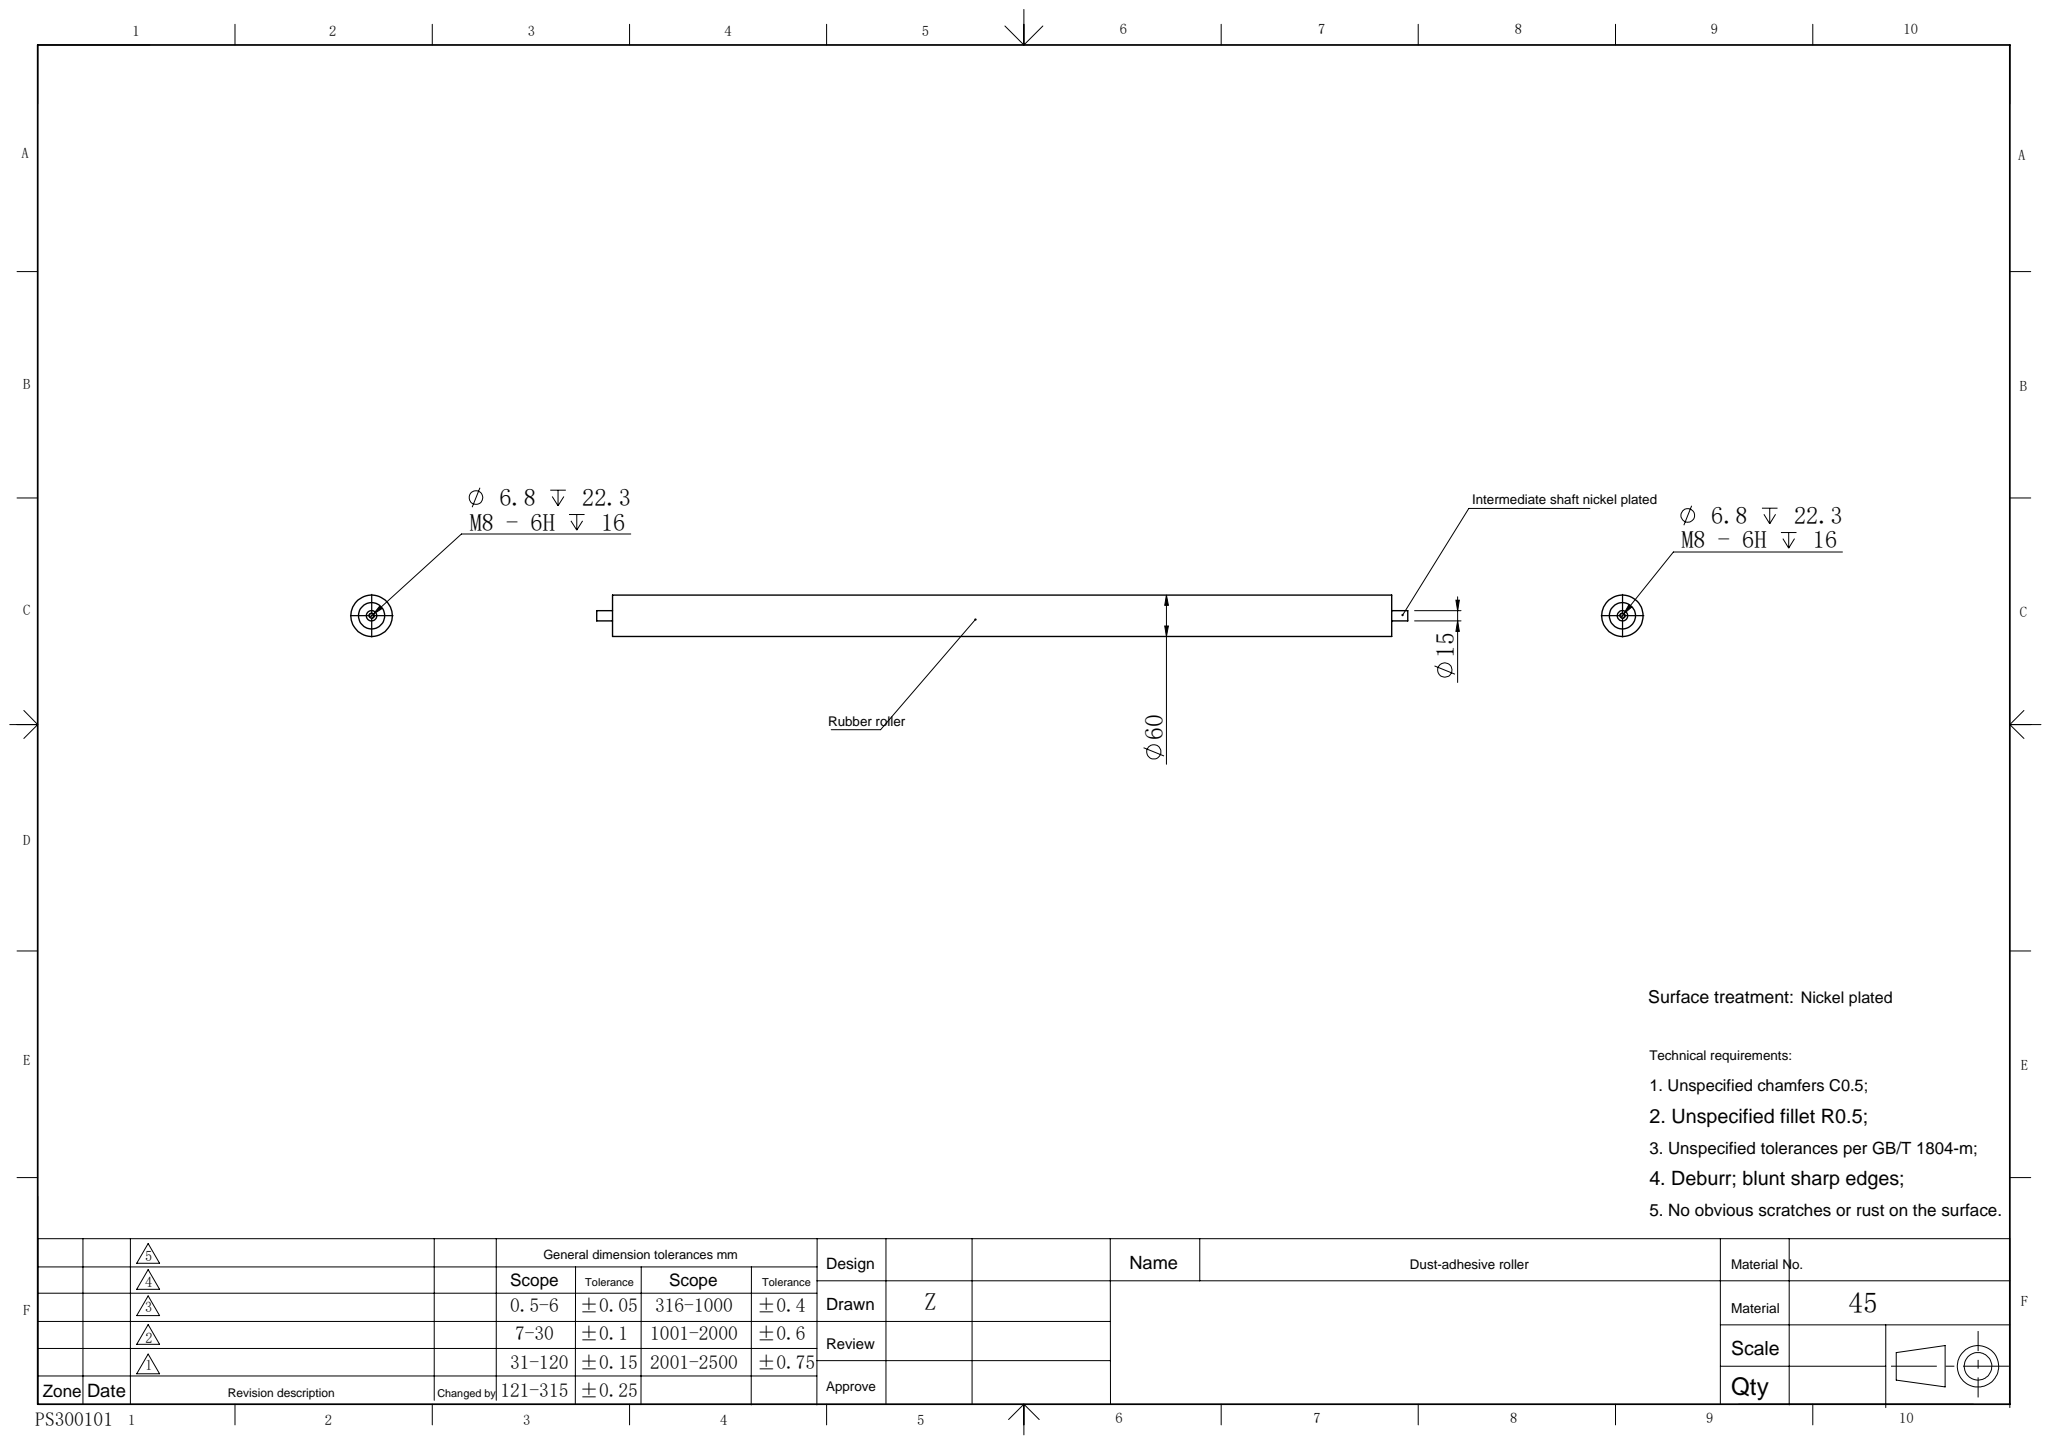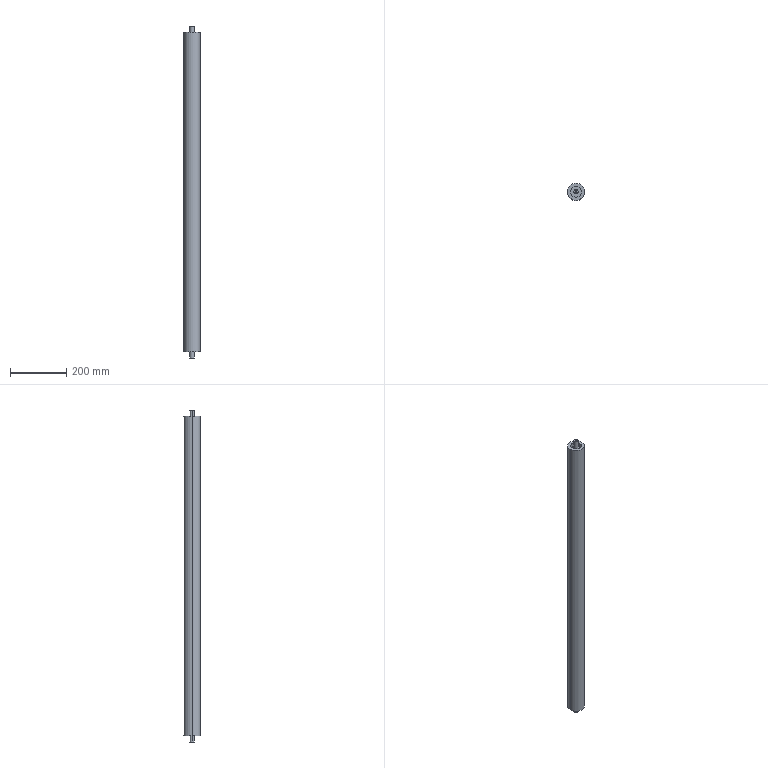Part | SolidWorks | features HoleWzd 2, ICE 2, Extrusion 1 | 2 solids | 24 faces | box 60 x 60 x 1176 mm | volume 3172741 mm3 | cylinder 14 | plane 6 | cone 4 | commonest cylinder face diameters 6.8 x4 15 x4 38 x4 60 x2
STEP:
#1=CARTESIAN_POINT('',(-19.,0.,565.));
#2=VERTEX_POINT('',#1);
#3=CARTESIAN_POINT('',(19.,0.,565.));
#4=VERTEX_POINT('',#3);
#5=CARTESIAN_POINT('',(0.,0.,565.));
#6=DIRECTION('',(0.,0.,1.));
#7=DIRECTION('',(1.,0.,0.));
#8=AXIS2_PLACEMENT_3D('',#5,#6,#7);
#9=CIRCLE('',#8,19.);
#10=EDGE_CURVE('',#2,#4,#9,.T.);
#11=ORIENTED_EDGE('',*,*,#10,.T.);
#12=CARTESIAN_POINT('',(19.,0.,-565.));
#13=VERTEX_POINT('',#12);
#14=CARTESIAN_POINT('',(19.,0.,565.));
#15=DIRECTION('',(0.,0.,-1.));
#16=VECTOR('',#15,1000.);
#17=LINE('',#14,#16);
#18=EDGE_CURVE('',#4,#13,#17,.T.);
#19=ORIENTED_EDGE('',*,*,#18,.T.);
#20=CARTESIAN_POINT('',(-19.,0.,-565.));
#21=VERTEX_POINT('',#20);
#22=CARTESIAN_POINT('',(0.,0.,-565.));
#23=DIRECTION('',(0.,0.,1.));
#24=DIRECTION('',(1.,0.,0.));
#25=AXIS2_PLACEMENT_3D('',#22,#23,#24);
#26=CIRCLE('',#25,19.);
#27=EDGE_CURVE('',#21,#13,#26,.T.);
#28=ORIENTED_EDGE('',*,*,#27,.F.);
#29=CARTESIAN_POINT('',(-19.,0.,565.));
#30=DIRECTION('',(0.,0.,-1.));
#31=VECTOR('',#30,1000.);
#32=LINE('',#29,#31);
#33=EDGE_CURVE('',#2,#21,#32,.T.);
#34=ORIENTED_EDGE('',*,*,#33,.F.);
#35=EDGE_LOOP('',(#11,#19,#28,#34));
#36=FACE_OUTER_BOUND('',#35,.T.);
#37=CARTESIAN_POINT('',(0.,0.,565.));
#38=DIRECTION('',(0.,0.,-1.));
#39=DIRECTION('',(-1.,0.,0.));
#40=AXIS2_PLACEMENT_3D('',#37,#38,#39);
#41=CYLINDRICAL_SURFACE('',#40,19.);
#42=ADVANCED_FACE('',(#36),#41,.F.);
#43=CARTESIAN_POINT('',(30.,0.,565.));
#44=VERTEX_POINT('',#43);
#45=CARTESIAN_POINT('',(-30.,0.,565.));
#46=VERTEX_POINT('',#45);
#47=CARTESIAN_POINT('',(0.,0.,565.));
#48=DIRECTION('',(0.,0.,1.));
#49=DIRECTION('',(1.,0.,0.));
#50=AXIS2_PLACEMENT_3D('',#47,#48,#49);
#51=CIRCLE('',#50,30.);
#52=EDGE_CURVE('',#44,#46,#51,.T.);
#53=ORIENTED_EDGE('',*,*,#52,.F.);
#54=CARTESIAN_POINT('',(30.,0.,-565.));
#55=VERTEX_POINT('',#54);
#56=CARTESIAN_POINT('',(30.,0.,565.));
#57=DIRECTION('',(0.,0.,-1.));
#58=VECTOR('',#57,1000.);
#59=LINE('',#56,#58);
#60=EDGE_CURVE('',#44,#55,#59,.T.);
#61=ORIENTED_EDGE('',*,*,#60,.T.);
#62=CARTESIAN_POINT('',(-30.,0.,-565.));
#63=VERTEX_POINT('',#62);
#64=CARTESIAN_POINT('',(0.,0.,-565.));
#65=DIRECTION('',(0.,0.,1.));
#66=DIRECTION('',(1.,0.,0.));
#67=AXIS2_PLACEMENT_3D('',#64,#65,#66);
#68=CIRCLE('',#67,30.);
#69=EDGE_CURVE('',#55,#63,#68,.T.);
#70=ORIENTED_EDGE('',*,*,#69,.T.);
#71=CARTESIAN_POINT('',(-30.,0.,565.));
#72=DIRECTION('',(0.,0.,-1.));
#73=VECTOR('',#72,1000.);
#74=LINE('',#71,#73);
#75=EDGE_CURVE('',#46,#63,#74,.T.);
#76=ORIENTED_EDGE('',*,*,#75,.F.);
#77=EDGE_LOOP('',(#53,#61,#70,#76));
#78=FACE_OUTER_BOUND('',#77,.T.);
#79=CARTESIAN_POINT('',(0.,0.,565.));
#80=DIRECTION('',(0.,0.,-1.));
#81=DIRECTION('',(-1.,0.,0.));
#82=AXIS2_PLACEMENT_3D('',#79,#80,#81);
#83=CYLINDRICAL_SURFACE('',#82,30.);
#84=ADVANCED_FACE('',(#78),#83,.T.);
#85=CARTESIAN_POINT('',(0.,0.,565.));
#86=DIRECTION('',(0.,0.,1.));
#87=DIRECTION('',(1.,0.,0.));
#88=AXIS2_PLACEMENT_3D('',#85,#86,#87);
#89=CIRCLE('',#88,30.);
#90=EDGE_CURVE('',#46,#44,#89,.T.);
#91=ORIENTED_EDGE('',*,*,#90,.T.);
#92=ORIENTED_EDGE('',*,*,#52,.T.);
#93=EDGE_LOOP('',(#91,#92));
#94=FACE_OUTER_BOUND('',#93,.T.);
#95=ORIENTED_EDGE('',*,*,#10,.F.);
#96=CARTESIAN_POINT('',(0.,0.,565.));
#97=DIRECTION('',(0.,0.,1.));
#98=DIRECTION('',(1.,0.,0.));
#99=AXIS2_PLACEMENT_3D('',#96,#97,#98);
#100=CIRCLE('',#99,19.);
#101=EDGE_CURVE('',#4,#2,#100,.T.);
#102=ORIENTED_EDGE('',*,*,#101,.F.);
#103=EDGE_LOOP('',(#95,#102));
#104=FACE_BOUND('',#103,.T.);
#105=CARTESIAN_POINT('',(0.,0.,565.));
#106=DIRECTION('',(0.,0.,1.));
#107=DIRECTION('',(1.,0.,0.));
#108=AXIS2_PLACEMENT_3D('',#105,#106,#107);
#109=PLANE('',#108);
#110=ADVANCED_FACE('',(#94,#104),#109,.T.);
#111=CARTESIAN_POINT('',(0.,0.,-565.));
#112=DIRECTION('',(0.,0.,1.));
#113=DIRECTION('',(1.,0.,0.));
#114=AXIS2_PLACEMENT_3D('',#111,#112,#113);
#115=CIRCLE('',#114,30.);
#116=EDGE_CURVE('',#63,#55,#115,.T.);
#117=ORIENTED_EDGE('',*,*,#116,.F.);
#118=ORIENTED_EDGE('',*,*,#69,.F.);
#119=EDGE_LOOP('',(#117,#118));
#120=FACE_OUTER_BOUND('',#119,.T.);
#121=ORIENTED_EDGE('',*,*,#27,.T.);
#122=CARTESIAN_POINT('',(0.,0.,-565.));
#123=DIRECTION('',(0.,0.,1.));
#124=DIRECTION('',(1.,0.,0.));
#125=AXIS2_PLACEMENT_3D('',#122,#123,#124);
#126=CIRCLE('',#125,19.);
#127=EDGE_CURVE('',#13,#21,#126,.T.);
#128=ORIENTED_EDGE('',*,*,#127,.T.);
#129=EDGE_LOOP('',(#121,#128));
#130=FACE_BOUND('',#129,.T.);
#131=CARTESIAN_POINT('',(0.,0.,-565.));
#132=DIRECTION('',(0.,0.,1.));
#133=DIRECTION('',(1.,0.,0.));
#134=AXIS2_PLACEMENT_3D('',#131,#132,#133);
#135=PLANE('',#134);
#136=ADVANCED_FACE('',(#120,#130),#135,.F.);
#137=ORIENTED_EDGE('',*,*,#60,.F.);
#138=ORIENTED_EDGE('',*,*,#90,.F.);
#139=ORIENTED_EDGE('',*,*,#75,.T.);
#140=ORIENTED_EDGE('',*,*,#116,.T.);
#141=EDGE_LOOP('',(#137,#138,#139,#140));
#142=FACE_OUTER_BOUND('',#141,.T.);
#143=CARTESIAN_POINT('',(0.,0.,565.));
#144=DIRECTION('',(0.,0.,-1.));
#145=DIRECTION('',(-1.,0.,0.));
#146=AXIS2_PLACEMENT_3D('',#143,#144,#145);
#147=CYLINDRICAL_SURFACE('',#146,30.);
#148=ADVANCED_FACE('',(#142),#147,.T.);
#149=ORIENTED_EDGE('',*,*,#18,.F.);
#150=ORIENTED_EDGE('',*,*,#101,.T.);
#151=ORIENTED_EDGE('',*,*,#33,.T.);
#152=ORIENTED_EDGE('',*,*,#127,.F.);
#153=EDGE_LOOP('',(#149,#150,#151,#152));
#154=FACE_OUTER_BOUND('',#153,.T.);
#155=CARTESIAN_POINT('',(0.,0.,565.));
#156=DIRECTION('',(0.,0.,-1.));
#157=DIRECTION('',(-1.,0.,0.));
#158=AXIS2_PLACEMENT_3D('',#155,#156,#157);
#159=CYLINDRICAL_SURFACE('',#158,19.);
#160=ADVANCED_FACE('',(#154),#159,.F.);
#161=CLOSED_SHELL('',(#42,#84,#110,#136,#148,#160));
#162=MANIFOLD_SOLID_BREP('',#161);
#163=CARTESIAN_POINT('',(-3.4,0.,565.75));
#164=VERTEX_POINT('',#163);
#165=CARTESIAN_POINT('',(3.4,0.,565.75));
#166=VERTEX_POINT('',#165);
#167=CARTESIAN_POINT('',(0.,0.,565.75));
#168=DIRECTION('',(0.,0.,1.));
#169=DIRECTION('',(1.,0.,0.));
#170=AXIS2_PLACEMENT_3D('',#167,#168,#169);
#171=CIRCLE('',#170,3.4);
#172=EDGE_CURVE('',#164,#166,#171,.T.);
#173=ORIENTED_EDGE('',*,*,#172,.F.);
#174=CARTESIAN_POINT('',(-3.4,0.,588.));
#175=VERTEX_POINT('',#174);
#176=CARTESIAN_POINT('',(-3.4,0.,588.));
#177=DIRECTION('',(0.,0.,1.));
#178=VECTOR('',#177,1000.);
#179=LINE('',#176,#178);
#180=EDGE_CURVE('',#164,#175,#179,.T.);
#181=ORIENTED_EDGE('',*,*,#180,.T.);
#182=CARTESIAN_POINT('',(3.4,0.,588.));
#183=VERTEX_POINT('',#182);
#184=CARTESIAN_POINT('',(0.,0.,588.));
#185=DIRECTION('',(0.,0.,1.));
#186=DIRECTION('',(1.,0.,0.));
#187=AXIS2_PLACEMENT_3D('',#184,#185,#186);
#188=CIRCLE('',#187,3.4);
#189=EDGE_CURVE('',#175,#183,#188,.T.);
#190=ORIENTED_EDGE('',*,*,#189,.T.);
#191=CARTESIAN_POINT('',(3.4,0.,588.));
#192=DIRECTION('',(0.,0.,1.));
#193=VECTOR('',#192,1000.);
#194=LINE('',#191,#193);
#195=EDGE_CURVE('',#166,#183,#194,.T.);
#196=ORIENTED_EDGE('',*,*,#195,.F.);
#197=EDGE_LOOP('',(#173,#181,#190,#196));
#198=FACE_OUTER_BOUND('',#197,.T.);
#199=CARTESIAN_POINT('',(0.,0.,588.));
#200=DIRECTION('',(0.,0.,1.));
#201=DIRECTION('',(1.,0.,0.));
#202=AXIS2_PLACEMENT_3D('',#199,#200,#201);
#203=CYLINDRICAL_SURFACE('',#202,3.4);
#204=ADVANCED_FACE('',(#198),#203,.F.);
#205=CARTESIAN_POINT('',(0.,0.,563.707));
#206=VERTEX_POINT('',#205);
#207=CARTESIAN_POINT('',(3.4,0.,565.75));
#208=DIRECTION('',(0.8572,0.,0.515));
#209=VECTOR('',#208,1000.);
#210=LINE('',#207,#209);
#211=EDGE_CURVE('',#206,#166,#210,.T.);
#212=ORIENTED_EDGE('',*,*,#211,.F.);
#213=CARTESIAN_POINT('',(-3.4,0.,565.75));
#214=DIRECTION('',(-0.8572,0.,0.515));
#215=VECTOR('',#214,1000.);
#216=LINE('',#213,#215);
#217=EDGE_CURVE('',#206,#164,#216,.T.);
#218=ORIENTED_EDGE('',*,*,#217,.T.);
#219=ORIENTED_EDGE('',*,*,#172,.T.);
#220=EDGE_LOOP('',(#212,#218,#219));
#221=FACE_OUTER_BOUND('',#220,.T.);
#222=CARTESIAN_POINT('',(0.,0.,565.75));
#223=DIRECTION('',(0.,0.,1.));
#224=DIRECTION('',(1.,0.,0.));
#225=AXIS2_PLACEMENT_3D('',#222,#223,#224);
#226=CONICAL_SURFACE('',#225,3.4,1.03);
#227=ADVANCED_FACE('',(#221),#226,.F.);
#228=CARTESIAN_POINT('',(3.4,0.,-565.75));
#229=VERTEX_POINT('',#228);
#230=CARTESIAN_POINT('',(-3.4,0.,-565.75));
#231=VERTEX_POINT('',#230);
#232=CARTESIAN_POINT('',(0.,0.,-565.75));
#233=DIRECTION('',(0.,0.,-1.));
#234=DIRECTION('',(-1.,0.,0.));
#235=AXIS2_PLACEMENT_3D('',#232,#233,#234);
#236=CIRCLE('',#235,3.4);
#237=EDGE_CURVE('',#229,#231,#236,.T.);
#238=ORIENTED_EDGE('',*,*,#237,.F.);
#239=CARTESIAN_POINT('',(3.4,0.,-588.));
#240=VERTEX_POINT('',#239);
#241=CARTESIAN_POINT('',(3.4,0.,-588.));
#242=DIRECTION('',(0.,0.,-1.));
#243=VECTOR('',#242,1000.);
#244=LINE('',#241,#243);
#245=EDGE_CURVE('',#229,#240,#244,.T.);
#246=ORIENTED_EDGE('',*,*,#245,.T.);
#247=CARTESIAN_POINT('',(-3.4,0.,-588.));
#248=VERTEX_POINT('',#247);
#249=CARTESIAN_POINT('',(0.,0.,-588.));
#250=DIRECTION('',(0.,0.,-1.));
#251=DIRECTION('',(-1.,0.,0.));
#252=AXIS2_PLACEMENT_3D('',#249,#250,#251);
#253=CIRCLE('',#252,3.4);
#254=EDGE_CURVE('',#240,#248,#253,.T.);
#255=ORIENTED_EDGE('',*,*,#254,.T.);
#256=CARTESIAN_POINT('',(-3.4,0.,-588.));
#257=DIRECTION('',(0.,0.,-1.));
#258=VECTOR('',#257,1000.);
#259=LINE('',#256,#258);
#260=EDGE_CURVE('',#231,#248,#259,.T.);
#261=ORIENTED_EDGE('',*,*,#260,.F.);
#262=EDGE_LOOP('',(#238,#246,#255,#261));
#263=FACE_OUTER_BOUND('',#262,.T.);
#264=CARTESIAN_POINT('',(0.,0.,-588.));
#265=DIRECTION('',(0.,0.,-1.));
#266=DIRECTION('',(-1.,0.,0.));
#267=AXIS2_PLACEMENT_3D('',#264,#265,#266);
#268=CYLINDRICAL_SURFACE('',#267,3.4);
#269=ADVANCED_FACE('',(#263),#268,.F.);
#270=CARTESIAN_POINT('',(0.,0.,-563.707));
#271=VERTEX_POINT('',#270);
#272=CARTESIAN_POINT('',(-3.4,0.,-565.75));
#273=DIRECTION('',(-0.8572,0.,-0.515));
#274=VECTOR('',#273,1000.);
#275=LINE('',#272,#274);
#276=EDGE_CURVE('',#271,#231,#275,.T.);
#277=ORIENTED_EDGE('',*,*,#276,.F.);
#278=CARTESIAN_POINT('',(3.4,0.,-565.75));
#279=DIRECTION('',(0.8572,0.,-0.515));
#280=VECTOR('',#279,1000.);
#281=LINE('',#278,#280);
#282=EDGE_CURVE('',#271,#229,#281,.T.);
#283=ORIENTED_EDGE('',*,*,#282,.T.);
#284=ORIENTED_EDGE('',*,*,#237,.T.);
#285=EDGE_LOOP('',(#277,#283,#284));
#286=FACE_OUTER_BOUND('',#285,.T.);
#287=CARTESIAN_POINT('',(0.,0.,-565.75));
#288=DIRECTION('',(0.,0.,-1.));
#289=DIRECTION('',(-1.,0.,0.));
#290=AXIS2_PLACEMENT_3D('',#287,#288,#289);
#291=CONICAL_SURFACE('',#290,3.4,1.03);
#292=ADVANCED_FACE('',(#286),#291,.F.);
#293=CARTESIAN_POINT('',(7.5,0.,-550.));
#294=VERTEX_POINT('',#293);
#295=CARTESIAN_POINT('',(-7.5,0.,-550.));
#296=VERTEX_POINT('',#295);
#297=CARTESIAN_POINT('',(0.,0.,-550.));
#298=DIRECTION('',(0.,0.,1.));
#299=DIRECTION('',(1.,0.,0.));
#300=AXIS2_PLACEMENT_3D('',#297,#298,#299);
#301=CIRCLE('',#300,7.5);
#302=EDGE_CURVE('',#294,#296,#301,.T.);
#303=ORIENTED_EDGE('',*,*,#302,.F.);
#304=CARTESIAN_POINT('',(7.5,0.,-588.));
#305=VERTEX_POINT('',#304);
#306=CARTESIAN_POINT('',(7.5,0.,588.));
#307=DIRECTION('',(0.,0.,-1.));
#308=VECTOR('',#307,1000.);
#309=LINE('',#306,#308);
#310=EDGE_CURVE('',#294,#305,#309,.T.);
#311=ORIENTED_EDGE('',*,*,#310,.T.);
#312=CARTESIAN_POINT('',(-7.5,0.,-588.));
#313=VERTEX_POINT('',#312);
#314=CARTESIAN_POINT('',(0.,0.,-588.));
#315=DIRECTION('',(0.,0.,1.));
#316=DIRECTION('',(1.,0.,0.));
#317=AXIS2_PLACEMENT_3D('',#314,#315,#316);
#318=CIRCLE('',#317,7.5);
#319=EDGE_CURVE('',#305,#313,#318,.T.);
#320=ORIENTED_EDGE('',*,*,#319,.T.);
#321=CARTESIAN_POINT('',(-7.5,0.,588.));
#322=DIRECTION('',(0.,0.,-1.));
#323=VECTOR('',#322,1000.);
#324=LINE('',#321,#323);
#325=EDGE_CURVE('',#296,#313,#324,.T.);
#326=ORIENTED_EDGE('',*,*,#325,.F.);
#327=EDGE_LOOP('',(#303,#311,#320,#326));
#328=FACE_OUTER_BOUND('',#327,.T.);
#329=CARTESIAN_POINT('',(0.,0.,588.));
#330=DIRECTION('',(0.,0.,-1.));
#331=DIRECTION('',(-1.,0.,0.));
#332=AXIS2_PLACEMENT_3D('',#329,#330,#331);
#333=CYLINDRICAL_SURFACE('',#332,7.5);
#334=ADVANCED_FACE('',(#328),#333,.T.);
#335=CARTESIAN_POINT('',(19.,0.,550.));
#336=VERTEX_POINT('',#335);
#337=CARTESIAN_POINT('',(-19.,0.,550.));
#338=VERTEX_POINT('',#337);
#339=CARTESIAN_POINT('',(0.,0.,550.));
#340=DIRECTION('',(0.,0.,1.));
#341=DIRECTION('',(1.,0.,0.));
#342=AXIS2_PLACEMENT_3D('',#339,#340,#341);
#343=CIRCLE('',#342,19.);
#344=EDGE_CURVE('',#336,#338,#343,.T.);
#345=ORIENTED_EDGE('',*,*,#344,.F.);
#346=CARTESIAN_POINT('',(19.,0.,-550.));
#347=VERTEX_POINT('',#346);
#348=CARTESIAN_POINT('',(19.,0.,550.));
#349=DIRECTION('',(0.,0.,-1.));
#350=VECTOR('',#349,1000.);
#351=LINE('',#348,#350);
#352=EDGE_CURVE('',#336,#347,#351,.T.);
#353=ORIENTED_EDGE('',*,*,#352,.T.);
#354=CARTESIAN_POINT('',(-19.,0.,-550.));
#355=VERTEX_POINT('',#354);
#356=CARTESIAN_POINT('',(0.,0.,-550.));
#357=DIRECTION('',(0.,0.,1.));
#358=DIRECTION('',(1.,0.,0.));
#359=AXIS2_PLACEMENT_3D('',#356,#357,#358);
#360=CIRCLE('',#359,19.);
#361=EDGE_CURVE('',#347,#355,#360,.T.);
#362=ORIENTED_EDGE('',*,*,#361,.T.);
#363=CARTESIAN_POINT('',(-19.,0.,550.));
#364=DIRECTION('',(0.,0.,-1.));
#365=VECTOR('',#364,1000.);
#366=LINE('',#363,#365);
#367=EDGE_CURVE('',#338,#355,#366,.T.);
#368=ORIENTED_EDGE('',*,*,#367,.F.);
#369=EDGE_LOOP('',(#345,#353,#362,#368));
#370=FACE_OUTER_BOUND('',#369,.T.);
#371=CARTESIAN_POINT('',(0.,0.,550.));
#372=DIRECTION('',(0.,0.,-1.));
#373=DIRECTION('',(-1.,0.,0.));
#374=AXIS2_PLACEMENT_3D('',#371,#372,#373);
#375=CYLINDRICAL_SURFACE('',#374,19.);
#376=ADVANCED_FACE('',(#370),#375,.T.);
#377=CARTESIAN_POINT('',(7.5,0.,588.));
#378=VERTEX_POINT('',#377);
#379=CARTESIAN_POINT('',(-7.5,0.,588.));
#380=VERTEX_POINT('',#379);
#381=CARTESIAN_POINT('',(0.,0.,588.));
#382=DIRECTION('',(0.,0.,1.));
#383=DIRECTION('',(1.,0.,0.));
#384=AXIS2_PLACEMENT_3D('',#381,#382,#383);
#385=CIRCLE('',#384,7.5);
#386=EDGE_CURVE('',#378,#380,#385,.T.);
#387=ORIENTED_EDGE('',*,*,#386,.F.);
#388=CARTESIAN_POINT('',(7.5,0.,550.));
#389=VERTEX_POINT('',#388);
#390=CARTESIAN_POINT('',(7.5,0.,588.));
#391=DIRECTION('',(0.,0.,-1.));
#392=VECTOR('',#391,1000.);
#393=LINE('',#390,#392);
#394=EDGE_CURVE('',#378,#389,#393,.T.);
#395=ORIENTED_EDGE('',*,*,#394,.T.);
#396=CARTESIAN_POINT('',(-7.5,0.,550.));
#397=VERTEX_POINT('',#396);
#398=CARTESIAN_POINT('',(0.,0.,550.));
#399=DIRECTION('',(0.,0.,1.));
#400=DIRECTION('',(1.,0.,0.));
#401=AXIS2_PLACEMENT_3D('',#398,#399,#400);
#402=CIRCLE('',#401,7.5);
#403=EDGE_CURVE('',#389,#397,#402,.T.);
#404=ORIENTED_EDGE('',*,*,#403,.T.);
#405=CARTESIAN_POINT('',(-7.5,0.,588.));
#406=DIRECTION('',(0.,0.,-1.));
#407=VECTOR('',#406,1000.);
#408=LINE('',#405,#407);
#409=EDGE_CURVE('',#380,#397,#408,.T.);
#410=ORIENTED_EDGE('',*,*,#409,.F.);
#411=EDGE_LOOP('',(#387,#395,#404,#410));
#412=FACE_OUTER_BOUND('',#411,.T.);
#413=CARTESIAN_POINT('',(0.,0.,588.));
#414=DIRECTION('',(0.,0.,-1.));
#415=DIRECTION('',(-1.,0.,0.));
#416=AXIS2_PLACEMENT_3D('',#413,#414,#415);
#417=CYLINDRICAL_SURFACE('',#416,7.5);
#418=ADVANCED_FACE('',(#412),#417,.T.);
#419=ORIENTED_EDGE('',*,*,#394,.F.);
#420=CARTESIAN_POINT('',(0.,0.,588.));
#421=DIRECTION('',(0.,0.,1.));
#422=DIRECTION('',(1.,0.,0.));
#423=AXIS2_PLACEMENT_3D('',#420,#421,#422);
#424=CIRCLE('',#423,7.5);
#425=EDGE_CURVE('',#380,#378,#424,.T.);
#426=ORIENTED_EDGE('',*,*,#425,.F.);
#427=ORIENTED_EDGE('',*,*,#409,.T.);
#428=CARTESIAN_POINT('',(0.,0.,550.));
#429=DIRECTION('',(0.,0.,1.));
#430=DIRECTION('',(1.,0.,0.));
#431=AXIS2_PLACEMENT_3D('',#428,#429,#430);
#432=CIRCLE('',#431,7.5);
#433=EDGE_CURVE('',#397,#389,#432,.T.);
#434=ORIENTED_EDGE('',*,*,#433,.T.);
#435=EDGE_LOOP('',(#419,#426,#427,#434));
#436=FACE_OUTER_BOUND('',#435,.T.);
#437=CARTESIAN_POINT('',(0.,0.,588.));
#438=DIRECTION('',(0.,0.,-1.));
#439=DIRECTION('',(-1.,0.,0.));
#440=AXIS2_PLACEMENT_3D('',#437,#438,#439);
#441=CYLINDRICAL_SURFACE('',#440,7.5);
#442=ADVANCED_FACE('',(#436),#441,.T.);
#443=CARTESIAN_POINT('',(0.,0.,588.));
#444=DIRECTION('',(0.,0.,1.));
#445=DIRECTION('',(1.,0.,0.));
#446=AXIS2_PLACEMENT_3D('',#443,#444,#445);
#447=CIRCLE('',#446,3.4);
#448=EDGE_CURVE('',#183,#175,#447,.T.);
#449=ORIENTED_EDGE('',*,*,#448,.F.);
#450=ORIENTED_EDGE('',*,*,#189,.F.);
#451=EDGE_LOOP('',(#449,#450));
#452=FACE_BOUND('',#451,.T.);
#453=ORIENTED_EDGE('',*,*,#425,.T.);
#454=ORIENTED_EDGE('',*,*,#386,.T.);
#455=EDGE_LOOP('',(#453,#454));
#456=FACE_OUTER_BOUND('',#455,.T.);
#457=CARTESIAN_POINT('',(0.,0.,588.));
#458=DIRECTION('',(0.,0.,1.));
#459=DIRECTION('',(1.,0.,0.));
#460=AXIS2_PLACEMENT_3D('',#457,#458,#459);
#461=PLANE('',#460);
#462=ADVANCED_FACE('',(#452,#456),#461,.T.);
#463=ORIENTED_EDGE('',*,*,#352,.F.);
#464=CARTESIAN_POINT('',(0.,0.,550.));
#465=DIRECTION('',(0.,0.,1.));
#466=DIRECTION('',(1.,0.,0.));
#467=AXIS2_PLACEMENT_3D('',#464,#465,#466);
#468=CIRCLE('',#467,19.);
#469=EDGE_CURVE('',#338,#336,#468,.T.);
#470=ORIENTED_EDGE('',*,*,#469,.F.);
#471=ORIENTED_EDGE('',*,*,#367,.T.);
#472=CARTESIAN_POINT('',(0.,0.,-550.));
#473=DIRECTION('',(0.,0.,1.));
#474=DIRECTION('',(1.,0.,0.));
#475=AXIS2_PLACEMENT_3D('',#472,#473,#474);
#476=CIRCLE('',#475,19.);
#477=EDGE_CURVE('',#355,#347,#476,.T.);
#478=ORIENTED_EDGE('',*,*,#477,.T.);
#479=EDGE_LOOP('',(#463,#470,#471,#478));
#480=FACE_OUTER_BOUND('',#479,.T.);
#481=CARTESIAN_POINT('',(0.,0.,550.));
#482=DIRECTION('',(0.,0.,-1.));
#483=DIRECTION('',(-1.,0.,0.));
#484=AXIS2_PLACEMENT_3D('',#481,#482,#483);
#485=CYLINDRICAL_SURFACE('',#484,19.);
#486=ADVANCED_FACE('',(#480),#485,.T.);
#487=ORIENTED_EDGE('',*,*,#433,.F.);
#488=ORIENTED_EDGE('',*,*,#403,.F.);
#489=EDGE_LOOP('',(#487,#488));
#490=FACE_BOUND('',#489,.T.);
#491=ORIENTED_EDGE('',*,*,#469,.T.);
#492=ORIENTED_EDGE('',*,*,#344,.T.);
#493=EDGE_LOOP('',(#491,#492));
#494=FACE_OUTER_BOUND('',#493,.T.);
#495=CARTESIAN_POINT('',(0.,0.,550.));
#496=DIRECTION('',(0.,0.,1.));
#497=DIRECTION('',(1.,0.,0.));
#498=AXIS2_PLACEMENT_3D('',#495,#496,#497);
#499=PLANE('',#498);
#500=ADVANCED_FACE('',(#490,#494),#499,.T.);
#501=CARTESIAN_POINT('',(0.,0.,-550.));
#502=DIRECTION('',(0.,0.,1.));
#503=DIRECTION('',(1.,0.,0.));
#504=AXIS2_PLACEMENT_3D('',#501,#502,#503);
#505=CIRCLE('',#504,7.5);
#506=EDGE_CURVE('',#296,#294,#505,.T.);
#507=ORIENTED_EDGE('',*,*,#506,.T.);
#508=ORIENTED_EDGE('',*,*,#302,.T.);
#509=EDGE_LOOP('',(#507,#508));
#510=FACE_BOUND('',#509,.T.);
#511=ORIENTED_EDGE('',*,*,#477,.F.);
#512=ORIENTED_EDGE('',*,*,#361,.F.);
#513=EDGE_LOOP('',(#511,#512));
#514=FACE_OUTER_BOUND('',#513,.T.);
#515=CARTESIAN_POINT('',(0.,0.,-550.));
#516=DIRECTION('',(0.,0.,1.));
#517=DIRECTION('',(1.,0.,0.));
#518=AXIS2_PLACEMENT_3D('',#515,#516,#517);
#519=PLANE('',#518);
#520=ADVANCED_FACE('',(#510,#514),#519,.F.);
#521=CARTESIAN_POINT('',(0.,0.,-588.));
#522=DIRECTION('',(0.,0.,-1.));
#523=DIRECTION('',(-1.,0.,0.));
#524=AXIS2_PLACEMENT_3D('',#521,#522,#523);
#525=CIRCLE('',#524,3.4);
#526=EDGE_CURVE('',#248,#240,#525,.T.);
#527=ORIENTED_EDGE('',*,*,#526,.F.);
#528=ORIENTED_EDGE('',*,*,#254,.F.);
#529=EDGE_LOOP('',(#527,#528));
#530=FACE_BOUND('',#529,.T.);
#531=CARTESIAN_POINT('',(0.,0.,-588.));
#532=DIRECTION('',(0.,0.,1.));
#533=DIRECTION('',(1.,0.,0.));
#534=AXIS2_PLACEMENT_3D('',#531,#532,#533);
#535=CIRCLE('',#534,7.5);
#536=EDGE_CURVE('',#313,#305,#535,.T.);
#537=ORIENTED_EDGE('',*,*,#536,.F.);
#538=ORIENTED_EDGE('',*,*,#319,.F.);
#539=EDGE_LOOP('',(#537,#538));
#540=FACE_OUTER_BOUND('',#539,.T.);
#541=CARTESIAN_POINT('',(0.,0.,-588.));
#542=DIRECTION('',(0.,0.,1.));
#543=DIRECTION('',(1.,0.,0.));
#544=AXIS2_PLACEMENT_3D('',#541,#542,#543);
#545=PLANE('',#544);
#546=ADVANCED_FACE('',(#530,#540),#545,.F.);
#547=ORIENTED_EDGE('',*,*,#310,.F.);
#548=ORIENTED_EDGE('',*,*,#506,.F.);
#549=ORIENTED_EDGE('',*,*,#325,.T.);
#550=ORIENTED_EDGE('',*,*,#536,.T.);
#551=EDGE_LOOP('',(#547,#548,#549,#550));
#552=FACE_OUTER_BOUND('',#551,.T.);
#553=CARTESIAN_POINT('',(0.,0.,588.));
#554=DIRECTION('',(0.,0.,-1.));
#555=DIRECTION('',(-1.,0.,0.));
#556=AXIS2_PLACEMENT_3D('',#553,#554,#555);
#557=CYLINDRICAL_SURFACE('',#556,7.5);
#558=ADVANCED_FACE('',(#552),#557,.T.);
#559=ORIENTED_EDGE('',*,*,#282,.F.);
#560=ORIENTED_EDGE('',*,*,#276,.T.);
#561=CARTESIAN_POINT('',(0.,0.,-565.75));
#562=DIRECTION('',(0.,0.,-1.));
#563=DIRECTION('',(-1.,0.,0.));
#564=AXIS2_PLACEMENT_3D('',#561,#562,#563);
#565=CIRCLE('',#564,3.4);
#566=EDGE_CURVE('',#231,#229,#565,.T.);
#567=ORIENTED_EDGE('',*,*,#566,.T.);
#568=EDGE_LOOP('',(#559,#560,#567));
#569=FACE_OUTER_BOUND('',#568,.T.);
#570=CARTESIAN_POINT('',(0.,0.,-565.75));
#571=DIRECTION('',(0.,0.,-1.));
#572=DIRECTION('',(-1.,0.,0.));
#573=AXIS2_PLACEMENT_3D('',#570,#571,#572);
#574=CONICAL_SURFACE('',#573,3.4,1.03);
#575=ADVANCED_FACE('',(#569),#574,.F.);
#576=ORIENTED_EDGE('',*,*,#245,.F.);
#577=ORIENTED_EDGE('',*,*,#566,.F.);
#578=ORIENTED_EDGE('',*,*,#260,.T.);
#579=ORIENTED_EDGE('',*,*,#526,.T.);
#580=EDGE_LOOP('',(#576,#577,#578,#579));
#581=FACE_OUTER_BOUND('',#580,.T.);
#582=CARTESIAN_POINT('',(0.,0.,-588.));
#583=DIRECTION('',(0.,0.,-1.));
#584=DIRECTION('',(-1.,0.,0.));
#585=AXIS2_PLACEMENT_3D('',#582,#583,#584);
#586=CYLINDRICAL_SURFACE('',#585,3.4);
#587=ADVANCED_FACE('',(#581),#586,.F.);
#588=ORIENTED_EDGE('',*,*,#217,.F.);
#589=ORIENTED_EDGE('',*,*,#211,.T.);
#590=CARTESIAN_POINT('',(0.,0.,565.75));
#591=DIRECTION('',(0.,0.,1.));
#592=DIRECTION('',(1.,0.,0.));
#593=AXIS2_PLACEMENT_3D('',#590,#591,#592);
#594=CIRCLE('',#593,3.4);
#595=EDGE_CURVE('',#166,#164,#594,.T.);
#596=ORIENTED_EDGE('',*,*,#595,.T.);
#597=EDGE_LOOP('',(#588,#589,#596));
#598=FACE_OUTER_BOUND('',#597,.T.);
#599=CARTESIAN_POINT('',(0.,0.,565.75));
#600=DIRECTION('',(0.,0.,1.));
#601=DIRECTION('',(1.,0.,0.));
#602=AXIS2_PLACEMENT_3D('',#599,#600,#601);
#603=CONICAL_SURFACE('',#602,3.4,1.03);
#604=ADVANCED_FACE('',(#598),#603,.F.);
#605=ORIENTED_EDGE('',*,*,#180,.F.);
#606=ORIENTED_EDGE('',*,*,#595,.F.);
#607=ORIENTED_EDGE('',*,*,#195,.T.);
#608=ORIENTED_EDGE('',*,*,#448,.T.);
#609=EDGE_LOOP('',(#605,#606,#607,#608));
#610=FACE_OUTER_BOUND('',#609,.T.);
#611=CARTESIAN_POINT('',(0.,0.,588.));
#612=DIRECTION('',(0.,0.,1.));
#613=DIRECTION('',(1.,0.,0.));
#614=AXIS2_PLACEMENT_3D('',#611,#612,#613);
#615=CYLINDRICAL_SURFACE('',#614,3.4);
#616=ADVANCED_FACE('',(#610),#615,.F.);
#617=CLOSED_SHELL('',(#204,#227,#269,#292,#334,#376,#418,#442,#462,#486,#500,#520,#546,#558,#575,#587,#604,#616));
#618=MANIFOLD_SOLID_BREP('',#617);
#619=CARTESIAN_POINT('',(0.,0.,0.));
#620=DIRECTION('',(0.,0.,1.));
#621=DIRECTION('',(1.,0.,0.));
#622=AXIS2_PLACEMENT_3D('',#619,#620,#621);
#623=(LENGTH_UNIT()NAMED_UNIT(*)SI_UNIT(.MILLI.,.METRE.));
#624=UNCERTAINTY_MEASURE_WITH_UNIT(LENGTH_MEASURE(0.00001),#623,'','');
#625=(NAMED_UNIT(*)PLANE_ANGLE_UNIT()SI_UNIT($,.RADIAN.));
#626=(NAMED_UNIT(*)SI_UNIT($,.STERADIAN.)SOLID_ANGLE_UNIT());
#627=(GEOMETRIC_REPRESENTATION_CONTEXT(3)GLOBAL_UNCERTAINTY_ASSIGNED_CONTEXT((#624))GLOBAL_UNIT_ASSIGNED_CONTEXT((#623,#625,#626))REPRESENTATION_CONTEXT('',''));
#628=ADVANCED_BREP_SHAPE_REPRESENTATION('',(#162,#618,#622),#627);